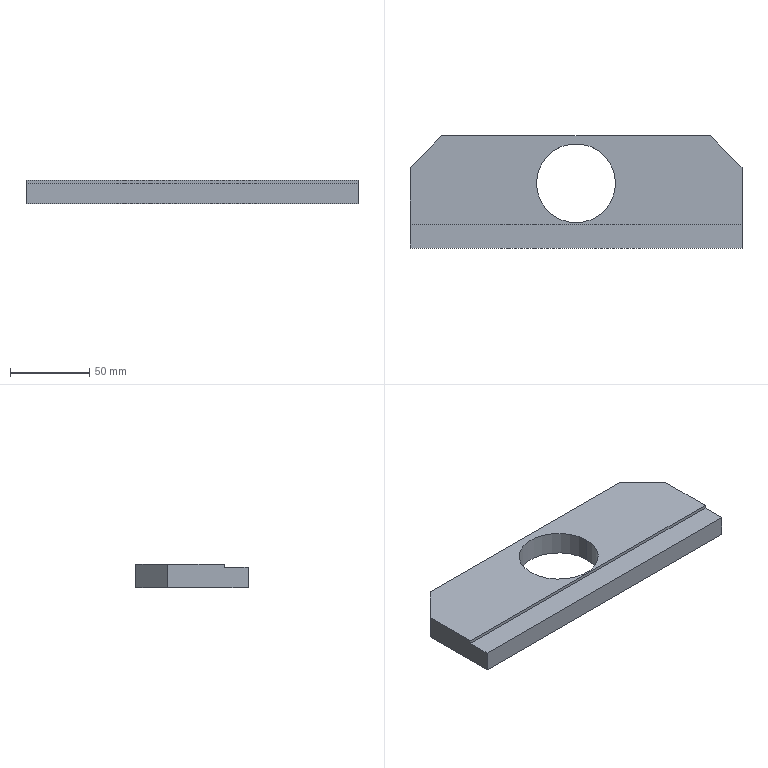Part | STEP file | 001-003-Shaft storage motor mounting plate | 1 solid | 12 faces | box 210 x 71 x 15 mm | volume 181898 mm3 | plane 10 | cylinder 2 | commonest cylinder face diameters 50 x2
STEP:
#1=CARTESIAN_POINT('',(0.,0.,0.));
#2=DIRECTION('',(0.,0.,1.));
#3=DIRECTION('',(1.,0.,0.));
#4=AXIS2_PLACEMENT_3D('',#1,#2,#3);
#5=CARTESIAN_POINT('',(-25.,5.5,15.));
#6=VERTEX_POINT('',#5);
#7=CARTESIAN_POINT('',(-25.,5.5,0.));
#8=VERTEX_POINT('',#7);
#9=CARTESIAN_POINT('',(-25.,5.5,15.));
#10=DIRECTION('',(0.,0.,-1.));
#11=VECTOR('',#10,1.);
#12=LINE('',#9,#11);
#13=CARTESIAN_POINT('',(0.,5.5,15.));
#14=DIRECTION('',(0.,0.,-1.));
#15=DIRECTION('',(-1.,0.,0.));
#16=AXIS2_PLACEMENT_3D('',#13,#14,#15);
#17=CYLINDRICAL_SURFACE('',#16,25.);
#18=CARTESIAN_POINT('',(6.283,0.));
#19=DIRECTION('',(0.,1.));
#20=VECTOR('',#19,1.);
#21=LINE('',#18,#20);
#22=(GEOMETRIC_REPRESENTATION_CONTEXT(2)PARAMETRIC_REPRESENTATION_CONTEXT()REPRESENTATION_CONTEXT('',''));
#23=DEFINITIONAL_REPRESENTATION('',(#21),#22);
#24=PCURVE('',#17,#23);
#25=CARTESIAN_POINT('',(0.,5.5,15.));
#26=DIRECTION('',(0.,0.,-1.));
#27=DIRECTION('',(-1.,0.,0.));
#28=AXIS2_PLACEMENT_3D('',#25,#26,#27);
#29=CYLINDRICAL_SURFACE('',#28,25.);
#30=CARTESIAN_POINT('',(0.,0.));
#31=DIRECTION('',(0.,1.));
#32=VECTOR('',#31,1.);
#33=LINE('',#30,#32);
#34=(GEOMETRIC_REPRESENTATION_CONTEXT(2)PARAMETRIC_REPRESENTATION_CONTEXT()REPRESENTATION_CONTEXT('',''));
#35=DEFINITIONAL_REPRESENTATION('',(#33),#34);
#36=PCURVE('',#29,#35);
#37=SURFACE_CURVE('',#12,(#24,#36),.PCURVE_S1.);
#38=EDGE_CURVE('',#6,#8,#37,.T.);
#39=ORIENTED_EDGE('',*,*,#38,.T.);
#40=CARTESIAN_POINT('',(25.,5.5,0.));
#41=VERTEX_POINT('',#40);
#42=CARTESIAN_POINT('',(0.,5.5,0.));
#43=DIRECTION('',(0.,0.,-1.));
#44=DIRECTION('',(-1.,0.,0.));
#45=AXIS2_PLACEMENT_3D('',#42,#43,#44);
#46=CIRCLE('',#45,25.);
#47=CARTESIAN_POINT('',(0.,15.));
#48=DIRECTION('',(1.,0.));
#49=VECTOR('',#48,1.);
#50=LINE('',#47,#49);
#51=(GEOMETRIC_REPRESENTATION_CONTEXT(2)PARAMETRIC_REPRESENTATION_CONTEXT()REPRESENTATION_CONTEXT('',''));
#52=DEFINITIONAL_REPRESENTATION('',(#50),#51);
#53=PCURVE('',#17,#52);
#54=CARTESIAN_POINT('',(0.,0.,0.));
#55=DIRECTION('',(0.,0.,-1.));
#56=DIRECTION('',(-1.,0.,0.));
#57=AXIS2_PLACEMENT_3D('',#54,#55,#56);
#58=PLANE('',#57);
#59=CARTESIAN_POINT('',(0.,5.5));
#60=DIRECTION('',(1.,0.));
#61=AXIS2_PLACEMENT_2D('',#59,#60);
#62=CIRCLE('',#61,25.);
#63=(GEOMETRIC_REPRESENTATION_CONTEXT(2)PARAMETRIC_REPRESENTATION_CONTEXT()REPRESENTATION_CONTEXT('',''));
#64=DEFINITIONAL_REPRESENTATION('',(#62),#63);
#65=PCURVE('',#58,#64);
#66=SURFACE_CURVE('',#46,(#53,#65),.PCURVE_S1.);
#67=EDGE_CURVE('',#41,#8,#66,.T.);
#68=ORIENTED_EDGE('',*,*,#67,.F.);
#69=CARTESIAN_POINT('',(25.,5.5,15.));
#70=VERTEX_POINT('',#69);
#71=CARTESIAN_POINT('',(25.,5.5,15.));
#72=DIRECTION('',(0.,0.,-1.));
#73=VECTOR('',#72,1.);
#74=LINE('',#71,#73);
#75=CARTESIAN_POINT('',(3.142,0.));
#76=DIRECTION('',(0.,1.));
#77=VECTOR('',#76,1.);
#78=LINE('',#75,#77);
#79=(GEOMETRIC_REPRESENTATION_CONTEXT(2)PARAMETRIC_REPRESENTATION_CONTEXT()REPRESENTATION_CONTEXT('',''));
#80=DEFINITIONAL_REPRESENTATION('',(#78),#79);
#81=PCURVE('',#17,#80);
#82=CARTESIAN_POINT('',(3.142,0.));
#83=DIRECTION('',(0.,1.));
#84=VECTOR('',#83,1.);
#85=LINE('',#82,#84);
#86=(GEOMETRIC_REPRESENTATION_CONTEXT(2)PARAMETRIC_REPRESENTATION_CONTEXT()REPRESENTATION_CONTEXT('',''));
#87=DEFINITIONAL_REPRESENTATION('',(#85),#86);
#88=PCURVE('',#29,#87);
#89=SURFACE_CURVE('',#74,(#81,#88),.PCURVE_S1.);
#90=EDGE_CURVE('',#70,#41,#89,.T.);
#91=ORIENTED_EDGE('',*,*,#90,.F.);
#92=CARTESIAN_POINT('',(0.,5.5,15.));
#93=DIRECTION('',(0.,0.,-1.));
#94=DIRECTION('',(-1.,0.,0.));
#95=AXIS2_PLACEMENT_3D('',#92,#93,#94);
#96=CIRCLE('',#95,25.);
#97=CARTESIAN_POINT('',(0.,0.));
#98=DIRECTION('',(1.,0.));
#99=VECTOR('',#98,1.);
#100=LINE('',#97,#99);
#101=(GEOMETRIC_REPRESENTATION_CONTEXT(2)PARAMETRIC_REPRESENTATION_CONTEXT()REPRESENTATION_CONTEXT('',''));
#102=DEFINITIONAL_REPRESENTATION('',(#100),#101);
#103=PCURVE('',#17,#102);
#104=CARTESIAN_POINT('',(0.,0.,15.));
#105=DIRECTION('',(0.,0.,-1.));
#106=DIRECTION('',(-1.,0.,0.));
#107=AXIS2_PLACEMENT_3D('',#104,#105,#106);
#108=PLANE('',#107);
#109=CARTESIAN_POINT('',(0.,5.5));
#110=DIRECTION('',(1.,0.));
#111=AXIS2_PLACEMENT_2D('',#109,#110);
#112=CIRCLE('',#111,25.);
#113=(GEOMETRIC_REPRESENTATION_CONTEXT(2)PARAMETRIC_REPRESENTATION_CONTEXT()REPRESENTATION_CONTEXT('',''));
#114=DEFINITIONAL_REPRESENTATION('',(#112),#113);
#115=PCURVE('',#108,#114);
#116=SURFACE_CURVE('',#96,(#103,#115),.PCURVE_S1.);
#117=EDGE_CURVE('',#70,#6,#116,.T.);
#118=ORIENTED_EDGE('',*,*,#117,.T.);
#119=EDGE_LOOP('',(#39,#68,#91,#118));
#120=FACE_BOUND('',#119,.F.);
#121=ADVANCED_FACE('',(#120),#17,.F.);
#122=CARTESIAN_POINT('',(-105.,-35.5,13.));
#123=VERTEX_POINT('',#122);
#124=CARTESIAN_POINT('',(105.,-35.5,13.));
#125=VERTEX_POINT('',#124);
#126=CARTESIAN_POINT('',(105.,-35.5,13.));
#127=DIRECTION('',(1.,0.,0.));
#128=VECTOR('',#127,1.);
#129=LINE('',#126,#128);
#130=CARTESIAN_POINT('',(-105.,-35.5,15.));
#131=DIRECTION('',(0.,1.,0.));
#132=DIRECTION('',(0.,0.,1.));
#133=AXIS2_PLACEMENT_3D('',#130,#131,#132);
#134=PLANE('',#133);
#135=CARTESIAN_POINT('',(-2.,210.));
#136=DIRECTION('',(0.,1.));
#137=VECTOR('',#136,1.);
#138=LINE('',#135,#137);
#139=(GEOMETRIC_REPRESENTATION_CONTEXT(2)PARAMETRIC_REPRESENTATION_CONTEXT()REPRESENTATION_CONTEXT('',''));
#140=DEFINITIONAL_REPRESENTATION('',(#138),#139);
#141=PCURVE('',#134,#140);
#142=CARTESIAN_POINT('',(0.,0.,13.));
#143=DIRECTION('',(0.,0.,1.));
#144=DIRECTION('',(1.,0.,0.));
#145=AXIS2_PLACEMENT_3D('',#142,#143,#144);
#146=PLANE('',#145);
#147=CARTESIAN_POINT('',(105.,-35.5));
#148=DIRECTION('',(1.,0.));
#149=VECTOR('',#148,1.);
#150=LINE('',#147,#149);
#151=(GEOMETRIC_REPRESENTATION_CONTEXT(2)PARAMETRIC_REPRESENTATION_CONTEXT()REPRESENTATION_CONTEXT('',''));
#152=DEFINITIONAL_REPRESENTATION('',(#150),#151);
#153=PCURVE('',#146,#152);
#154=SURFACE_CURVE('',#129,(#141,#153),.PCURVE_S1.);
#155=EDGE_CURVE('',#123,#125,#154,.T.);
#156=ORIENTED_EDGE('',*,*,#155,.F.);
#157=CARTESIAN_POINT('',(-105.,-35.5,0.));
#158=VERTEX_POINT('',#157);
#159=CARTESIAN_POINT('',(-105.,-35.5,15.));
#160=DIRECTION('',(0.,0.,-1.));
#161=VECTOR('',#160,1.);
#162=LINE('',#159,#161);
#163=CARTESIAN_POINT('',(0.,0.));
#164=DIRECTION('',(-1.,0.));
#165=VECTOR('',#164,1.);
#166=LINE('',#163,#165);
#167=(GEOMETRIC_REPRESENTATION_CONTEXT(2)PARAMETRIC_REPRESENTATION_CONTEXT()REPRESENTATION_CONTEXT('',''));
#168=DEFINITIONAL_REPRESENTATION('',(#166),#167);
#169=PCURVE('',#134,#168);
#170=CARTESIAN_POINT('',(-105.,-35.5,15.));
#171=DIRECTION('',(1.,0.,0.));
#172=DIRECTION('',(0.,0.,-1.));
#173=AXIS2_PLACEMENT_3D('',#170,#171,#172);
#174=PLANE('',#173);
#175=CARTESIAN_POINT('',(0.,0.));
#176=DIRECTION('',(1.,0.));
#177=VECTOR('',#176,1.);
#178=LINE('',#175,#177);
#179=(GEOMETRIC_REPRESENTATION_CONTEXT(2)PARAMETRIC_REPRESENTATION_CONTEXT()REPRESENTATION_CONTEXT('',''));
#180=DEFINITIONAL_REPRESENTATION('',(#178),#179);
#181=PCURVE('',#174,#180);
#182=SURFACE_CURVE('',#162,(#169,#181),.PCURVE_S1.);
#183=EDGE_CURVE('',#123,#158,#182,.T.);
#184=ORIENTED_EDGE('',*,*,#183,.T.);
#185=CARTESIAN_POINT('',(105.,-35.5,0.));
#186=VERTEX_POINT('',#185);
#187=CARTESIAN_POINT('',(-105.,-35.5,0.));
#188=DIRECTION('',(1.,0.,0.));
#189=VECTOR('',#188,1.);
#190=LINE('',#187,#189);
#191=CARTESIAN_POINT('',(-15.,0.));
#192=DIRECTION('',(0.,1.));
#193=VECTOR('',#192,1.);
#194=LINE('',#191,#193);
#195=(GEOMETRIC_REPRESENTATION_CONTEXT(2)PARAMETRIC_REPRESENTATION_CONTEXT()REPRESENTATION_CONTEXT('',''));
#196=DEFINITIONAL_REPRESENTATION('',(#194),#195);
#197=PCURVE('',#134,#196);
#198=CARTESIAN_POINT('',(105.,-35.5));
#199=DIRECTION('',(-1.,0.));
#200=VECTOR('',#199,1.);
#201=LINE('',#198,#200);
#202=(GEOMETRIC_REPRESENTATION_CONTEXT(2)PARAMETRIC_REPRESENTATION_CONTEXT()REPRESENTATION_CONTEXT('',''));
#203=DEFINITIONAL_REPRESENTATION('',(#201),#202);
#204=PCURVE('',#58,#203);
#205=SURFACE_CURVE('',#190,(#197,#204),.PCURVE_S1.);
#206=EDGE_CURVE('',#158,#186,#205,.T.);
#207=ORIENTED_EDGE('',*,*,#206,.T.);
#208=CARTESIAN_POINT('',(105.,-35.5,15.));
#209=DIRECTION('',(0.,0.,-1.));
#210=VECTOR('',#209,1.);
#211=LINE('',#208,#210);
#212=CARTESIAN_POINT('',(0.,210.));
#213=DIRECTION('',(-1.,0.));
#214=VECTOR('',#213,1.);
#215=LINE('',#212,#214);
#216=(GEOMETRIC_REPRESENTATION_CONTEXT(2)PARAMETRIC_REPRESENTATION_CONTEXT()REPRESENTATION_CONTEXT('',''));
#217=DEFINITIONAL_REPRESENTATION('',(#215),#216);
#218=PCURVE('',#134,#217);
#219=CARTESIAN_POINT('',(105.,-35.5,15.));
#220=DIRECTION('',(-1.,0.,0.));
#221=DIRECTION('',(0.,0.,1.));
#222=AXIS2_PLACEMENT_3D('',#219,#220,#221);
#223=PLANE('',#222);
#224=CARTESIAN_POINT('',(0.,0.));
#225=DIRECTION('',(-1.,0.));
#226=VECTOR('',#225,1.);
#227=LINE('',#224,#226);
#228=(GEOMETRIC_REPRESENTATION_CONTEXT(2)PARAMETRIC_REPRESENTATION_CONTEXT()REPRESENTATION_CONTEXT('',''));
#229=DEFINITIONAL_REPRESENTATION('',(#227),#228);
#230=PCURVE('',#223,#229);
#231=SURFACE_CURVE('',#211,(#218,#230),.PCURVE_S1.);
#232=EDGE_CURVE('',#125,#186,#231,.T.);
#233=ORIENTED_EDGE('',*,*,#232,.F.);
#234=EDGE_LOOP('',(#156,#184,#207,#233));
#235=FACE_BOUND('',#234,.T.);
#236=ADVANCED_FACE('',(#235),#134,.F.);
#237=CARTESIAN_POINT('',(105.,-20.5,15.));
#238=VERTEX_POINT('',#237);
#239=CARTESIAN_POINT('',(105.,15.5,15.));
#240=VERTEX_POINT('',#239);
#241=CARTESIAN_POINT('',(105.,-35.5,15.));
#242=DIRECTION('',(0.,1.,0.));
#243=VECTOR('',#242,1.);
#244=LINE('',#241,#243);
#245=CARTESIAN_POINT('',(0.,0.));
#246=DIRECTION('',(0.,1.));
#247=VECTOR('',#246,1.);
#248=LINE('',#245,#247);
#249=(GEOMETRIC_REPRESENTATION_CONTEXT(2)PARAMETRIC_REPRESENTATION_CONTEXT()REPRESENTATION_CONTEXT('',''));
#250=DEFINITIONAL_REPRESENTATION('',(#248),#249);
#251=PCURVE('',#223,#250);
#252=CARTESIAN_POINT('',(-105.,-35.5));
#253=DIRECTION('',(0.,1.));
#254=VECTOR('',#253,1.);
#255=LINE('',#252,#254);
#256=(GEOMETRIC_REPRESENTATION_CONTEXT(2)PARAMETRIC_REPRESENTATION_CONTEXT()REPRESENTATION_CONTEXT('',''));
#257=DEFINITIONAL_REPRESENTATION('',(#255),#256);
#258=PCURVE('',#108,#257);
#259=SURFACE_CURVE('',#244,(#251,#258),.PCURVE_S1.);
#260=EDGE_CURVE('',#238,#240,#259,.T.);
#261=ORIENTED_EDGE('',*,*,#260,.F.);
#262=CARTESIAN_POINT('',(105.,-20.5,13.));
#263=VERTEX_POINT('',#262);
#264=CARTESIAN_POINT('',(105.,-20.5,13.));
#265=DIRECTION('',(0.,0.,1.));
#266=VECTOR('',#265,1.);
#267=LINE('',#264,#266);
#268=CARTESIAN_POINT('',(-2.,15.));
#269=DIRECTION('',(1.,0.));
#270=VECTOR('',#269,1.);
#271=LINE('',#268,#270);
#272=(GEOMETRIC_REPRESENTATION_CONTEXT(2)PARAMETRIC_REPRESENTATION_CONTEXT()REPRESENTATION_CONTEXT('',''));
#273=DEFINITIONAL_REPRESENTATION('',(#271),#272);
#274=PCURVE('',#223,#273);
#275=CARTESIAN_POINT('',(105.,-20.5,13.));
#276=DIRECTION('',(0.,1.,0.));
#277=DIRECTION('',(-1.,0.,0.));
#278=AXIS2_PLACEMENT_3D('',#275,#276,#277);
#279=PLANE('',#278);
#280=CARTESIAN_POINT('',(0.,0.));
#281=DIRECTION('',(0.,1.));
#282=VECTOR('',#281,1.);
#283=LINE('',#280,#282);
#284=(GEOMETRIC_REPRESENTATION_CONTEXT(2)PARAMETRIC_REPRESENTATION_CONTEXT()REPRESENTATION_CONTEXT('',''));
#285=DEFINITIONAL_REPRESENTATION('',(#283),#284);
#286=PCURVE('',#279,#285);
#287=SURFACE_CURVE('',#267,(#274,#286),.PCURVE_S1.);
#288=EDGE_CURVE('',#263,#238,#287,.T.);
#289=ORIENTED_EDGE('',*,*,#288,.F.);
#290=CARTESIAN_POINT('',(105.,-35.5,13.));
#291=DIRECTION('',(0.,1.,0.));
#292=VECTOR('',#291,1.);
#293=LINE('',#290,#292);
#294=CARTESIAN_POINT('',(-2.,0.));
#295=DIRECTION('',(0.,1.));
#296=VECTOR('',#295,1.);
#297=LINE('',#294,#296);
#298=(GEOMETRIC_REPRESENTATION_CONTEXT(2)PARAMETRIC_REPRESENTATION_CONTEXT()REPRESENTATION_CONTEXT('',''));
#299=DEFINITIONAL_REPRESENTATION('',(#297),#298);
#300=PCURVE('',#223,#299);
#301=CARTESIAN_POINT('',(105.,-35.5));
#302=DIRECTION('',(0.,1.));
#303=VECTOR('',#302,1.);
#304=LINE('',#301,#303);
#305=(GEOMETRIC_REPRESENTATION_CONTEXT(2)PARAMETRIC_REPRESENTATION_CONTEXT()REPRESENTATION_CONTEXT('',''));
#306=DEFINITIONAL_REPRESENTATION('',(#304),#305);
#307=PCURVE('',#146,#306);
#308=SURFACE_CURVE('',#293,(#300,#307),.PCURVE_S1.);
#309=EDGE_CURVE('',#125,#263,#308,.T.);
#310=ORIENTED_EDGE('',*,*,#309,.F.);
#311=ORIENTED_EDGE('',*,*,#232,.T.);
#312=CARTESIAN_POINT('',(105.,15.5,0.));
#313=VERTEX_POINT('',#312);
#314=CARTESIAN_POINT('',(105.,-35.5,0.));
#315=DIRECTION('',(0.,1.,0.));
#316=VECTOR('',#315,1.);
#317=LINE('',#314,#316);
#318=CARTESIAN_POINT('',(-15.,0.));
#319=DIRECTION('',(0.,1.));
#320=VECTOR('',#319,1.);
#321=LINE('',#318,#320);
#322=(GEOMETRIC_REPRESENTATION_CONTEXT(2)PARAMETRIC_REPRESENTATION_CONTEXT()REPRESENTATION_CONTEXT('',''));
#323=DEFINITIONAL_REPRESENTATION('',(#321),#322);
#324=PCURVE('',#223,#323);
#325=CARTESIAN_POINT('',(-105.,-35.5));
#326=DIRECTION('',(0.,1.));
#327=VECTOR('',#326,1.);
#328=LINE('',#325,#327);
#329=(GEOMETRIC_REPRESENTATION_CONTEXT(2)PARAMETRIC_REPRESENTATION_CONTEXT()REPRESENTATION_CONTEXT('',''));
#330=DEFINITIONAL_REPRESENTATION('',(#328),#329);
#331=PCURVE('',#58,#330);
#332=SURFACE_CURVE('',#317,(#324,#331),.PCURVE_S1.);
#333=EDGE_CURVE('',#186,#313,#332,.T.);
#334=ORIENTED_EDGE('',*,*,#333,.T.);
#335=CARTESIAN_POINT('',(105.,15.5,15.));
#336=DIRECTION('',(0.,0.,1.));
#337=VECTOR('',#336,1.);
#338=LINE('',#335,#337);
#339=CARTESIAN_POINT('',(0.,51.));
#340=DIRECTION('',(1.,0.));
#341=VECTOR('',#340,1.);
#342=LINE('',#339,#341);
#343=(GEOMETRIC_REPRESENTATION_CONTEXT(2)PARAMETRIC_REPRESENTATION_CONTEXT()REPRESENTATION_CONTEXT('',''));
#344=DEFINITIONAL_REPRESENTATION('',(#342),#343);
#345=PCURVE('',#223,#344);
#346=CARTESIAN_POINT('',(85.,35.5,15.));
#347=DIRECTION('',(-0.7071,-0.7071,0.));
#348=DIRECTION('',(0.,0.,-1.));
#349=AXIS2_PLACEMENT_3D('',#346,#347,#348);
#350=PLANE('',#349);
#351=CARTESIAN_POINT('',(0.,28.284));
#352=DIRECTION('',(-1.,0.));
#353=VECTOR('',#352,1.);
#354=LINE('',#351,#353);
#355=(GEOMETRIC_REPRESENTATION_CONTEXT(2)PARAMETRIC_REPRESENTATION_CONTEXT()REPRESENTATION_CONTEXT('',''));
#356=DEFINITIONAL_REPRESENTATION('',(#354),#355);
#357=PCURVE('',#350,#356);
#358=SURFACE_CURVE('',#338,(#345,#357),.PCURVE_S1.);
#359=EDGE_CURVE('',#313,#240,#358,.T.);
#360=ORIENTED_EDGE('',*,*,#359,.T.);
#361=EDGE_LOOP('',(#261,#289,#310,#311,#334,#360));
#362=FACE_BOUND('',#361,.T.);
#363=ADVANCED_FACE('',(#362),#223,.F.);
#364=CARTESIAN_POINT('',(85.,35.5,0.));
#365=VERTEX_POINT('',#364);
#366=CARTESIAN_POINT('',(-85.,35.5,0.));
#367=VERTEX_POINT('',#366);
#368=CARTESIAN_POINT('',(-105.,35.5,0.));
#369=DIRECTION('',(-1.,0.,0.));
#370=VECTOR('',#369,1.);
#371=LINE('',#368,#370);
#372=CARTESIAN_POINT('',(-105.,35.5,15.));
#373=DIRECTION('',(0.,-1.,0.));
#374=DIRECTION('',(0.,0.,-1.));
#375=AXIS2_PLACEMENT_3D('',#372,#373,#374);
#376=PLANE('',#375);
#377=CARTESIAN_POINT('',(15.,0.));
#378=DIRECTION('',(0.,-1.));
#379=VECTOR('',#378,1.);
#380=LINE('',#377,#379);
#381=(GEOMETRIC_REPRESENTATION_CONTEXT(2)PARAMETRIC_REPRESENTATION_CONTEXT()REPRESENTATION_CONTEXT('',''));
#382=DEFINITIONAL_REPRESENTATION('',(#380),#381);
#383=PCURVE('',#376,#382);
#384=CARTESIAN_POINT('',(105.,35.5));
#385=DIRECTION('',(1.,0.));
#386=VECTOR('',#385,1.);
#387=LINE('',#384,#386);
#388=(GEOMETRIC_REPRESENTATION_CONTEXT(2)PARAMETRIC_REPRESENTATION_CONTEXT()REPRESENTATION_CONTEXT('',''));
#389=DEFINITIONAL_REPRESENTATION('',(#387),#388);
#390=PCURVE('',#58,#389);
#391=SURFACE_CURVE('',#371,(#383,#390),.PCURVE_S1.);
#392=EDGE_CURVE('',#365,#367,#391,.T.);
#393=ORIENTED_EDGE('',*,*,#392,.T.);
#394=CARTESIAN_POINT('',(-85.,35.5,15.));
#395=VERTEX_POINT('',#394);
#396=CARTESIAN_POINT('',(-85.,35.5,15.));
#397=DIRECTION('',(0.,0.,1.));
#398=VECTOR('',#397,1.);
#399=LINE('',#396,#398);
#400=CARTESIAN_POINT('',(0.,20.));
#401=DIRECTION('',(-1.,0.));
#402=VECTOR('',#401,1.);
#403=LINE('',#400,#402);
#404=(GEOMETRIC_REPRESENTATION_CONTEXT(2)PARAMETRIC_REPRESENTATION_CONTEXT()REPRESENTATION_CONTEXT('',''));
#405=DEFINITIONAL_REPRESENTATION('',(#403),#404);
#406=PCURVE('',#376,#405);
#407=CARTESIAN_POINT('',(-105.,15.5,15.));
#408=DIRECTION('',(0.7071,-0.7071,0.));
#409=DIRECTION('',(0.,0.,-1.));
#410=AXIS2_PLACEMENT_3D('',#407,#408,#409);
#411=PLANE('',#410);
#412=CARTESIAN_POINT('',(0.,28.284));
#413=DIRECTION('',(-1.,0.));
#414=VECTOR('',#413,1.);
#415=LINE('',#412,#414);
#416=(GEOMETRIC_REPRESENTATION_CONTEXT(2)PARAMETRIC_REPRESENTATION_CONTEXT()REPRESENTATION_CONTEXT('',''));
#417=DEFINITIONAL_REPRESENTATION('',(#415),#416);
#418=PCURVE('',#411,#417);
#419=SURFACE_CURVE('',#399,(#406,#418),.PCURVE_S1.);
#420=EDGE_CURVE('',#367,#395,#419,.T.);
#421=ORIENTED_EDGE('',*,*,#420,.T.);
#422=CARTESIAN_POINT('',(85.,35.5,15.));
#423=VERTEX_POINT('',#422);
#424=CARTESIAN_POINT('',(-105.,35.5,15.));
#425=DIRECTION('',(-1.,0.,0.));
#426=VECTOR('',#425,1.);
#427=LINE('',#424,#426);
#428=CARTESIAN_POINT('',(0.,0.));
#429=DIRECTION('',(0.,-1.));
#430=VECTOR('',#429,1.);
#431=LINE('',#428,#430);
#432=(GEOMETRIC_REPRESENTATION_CONTEXT(2)PARAMETRIC_REPRESENTATION_CONTEXT()REPRESENTATION_CONTEXT('',''));
#433=DEFINITIONAL_REPRESENTATION('',(#431),#432);
#434=PCURVE('',#376,#433);
#435=CARTESIAN_POINT('',(105.,35.5));
#436=DIRECTION('',(1.,0.));
#437=VECTOR('',#436,1.);
#438=LINE('',#435,#437);
#439=(GEOMETRIC_REPRESENTATION_CONTEXT(2)PARAMETRIC_REPRESENTATION_CONTEXT()REPRESENTATION_CONTEXT('',''));
#440=DEFINITIONAL_REPRESENTATION('',(#438),#439);
#441=PCURVE('',#108,#440);
#442=SURFACE_CURVE('',#427,(#434,#441),.PCURVE_S1.);
#443=EDGE_CURVE('',#423,#395,#442,.T.);
#444=ORIENTED_EDGE('',*,*,#443,.F.);
#445=CARTESIAN_POINT('',(85.,35.5,15.));
#446=DIRECTION('',(0.,0.,-1.));
#447=VECTOR('',#446,1.);
#448=LINE('',#445,#447);
#449=CARTESIAN_POINT('',(0.,190.));
#450=DIRECTION('',(1.,0.));
#451=VECTOR('',#450,1.);
#452=LINE('',#449,#451);
#453=(GEOMETRIC_REPRESENTATION_CONTEXT(2)PARAMETRIC_REPRESENTATION_CONTEXT()REPRESENTATION_CONTEXT('',''));
#454=DEFINITIONAL_REPRESENTATION('',(#452),#453);
#455=PCURVE('',#376,#454);
#456=CARTESIAN_POINT('',(0.,0.));
#457=DIRECTION('',(1.,0.));
#458=VECTOR('',#457,1.);
#459=LINE('',#456,#458);
#460=(GEOMETRIC_REPRESENTATION_CONTEXT(2)PARAMETRIC_REPRESENTATION_CONTEXT()REPRESENTATION_CONTEXT('',''));
#461=DEFINITIONAL_REPRESENTATION('',(#459),#460);
#462=PCURVE('',#350,#461);
#463=SURFACE_CURVE('',#448,(#455,#462),.PCURVE_S1.);
#464=EDGE_CURVE('',#423,#365,#463,.T.);
#465=ORIENTED_EDGE('',*,*,#464,.T.);
#466=EDGE_LOOP('',(#393,#421,#444,#465));
#467=FACE_BOUND('',#466,.T.);
#468=ADVANCED_FACE('',(#467),#376,.F.);
#469=CARTESIAN_POINT('',(-105.,-20.5,13.));
#470=VERTEX_POINT('',#469);
#471=CARTESIAN_POINT('',(-105.,-35.5,13.));
#472=DIRECTION('',(0.,-1.,0.));
#473=VECTOR('',#472,1.);
#474=LINE('',#471,#473);
#475=CARTESIAN_POINT('',(2.,0.));
#476=DIRECTION('',(0.,-1.));
#477=VECTOR('',#476,1.);
#478=LINE('',#475,#477);
#479=(GEOMETRIC_REPRESENTATION_CONTEXT(2)PARAMETRIC_REPRESENTATION_CONTEXT()REPRESENTATION_CONTEXT('',''));
#480=DEFINITIONAL_REPRESENTATION('',(#478),#479);
#481=PCURVE('',#174,#480);
#482=CARTESIAN_POINT('',(-105.,-35.5));
#483=DIRECTION('',(0.,-1.));
#484=VECTOR('',#483,1.);
#485=LINE('',#482,#484);
#486=(GEOMETRIC_REPRESENTATION_CONTEXT(2)PARAMETRIC_REPRESENTATION_CONTEXT()REPRESENTATION_CONTEXT('',''));
#487=DEFINITIONAL_REPRESENTATION('',(#485),#486);
#488=PCURVE('',#146,#487);
#489=SURFACE_CURVE('',#474,(#481,#488),.PCURVE_S1.);
#490=EDGE_CURVE('',#470,#123,#489,.T.);
#491=ORIENTED_EDGE('',*,*,#490,.F.);
#492=CARTESIAN_POINT('',(-105.,-20.5,15.));
#493=VERTEX_POINT('',#492);
#494=CARTESIAN_POINT('',(-105.,-20.5,13.));
#495=DIRECTION('',(0.,0.,1.));
#496=VECTOR('',#495,1.);
#497=LINE('',#494,#496);
#498=CARTESIAN_POINT('',(2.,15.));
#499=DIRECTION('',(-1.,0.));
#500=VECTOR('',#499,1.);
#501=LINE('',#498,#500);
#502=(GEOMETRIC_REPRESENTATION_CONTEXT(2)PARAMETRIC_REPRESENTATION_CONTEXT()REPRESENTATION_CONTEXT('',''));
#503=DEFINITIONAL_REPRESENTATION('',(#501),#502);
#504=PCURVE('',#174,#503);
#505=CARTESIAN_POINT('',(210.,0.));
#506=DIRECTION('',(0.,1.));
#507=VECTOR('',#506,1.);
#508=LINE('',#505,#507);
#509=(GEOMETRIC_REPRESENTATION_CONTEXT(2)PARAMETRIC_REPRESENTATION_CONTEXT()REPRESENTATION_CONTEXT('',''));
#510=DEFINITIONAL_REPRESENTATION('',(#508),#509);
#511=PCURVE('',#279,#510);
#512=SURFACE_CURVE('',#497,(#504,#511),.PCURVE_S1.);
#513=EDGE_CURVE('',#470,#493,#512,.T.);
#514=ORIENTED_EDGE('',*,*,#513,.T.);
#515=CARTESIAN_POINT('',(-105.,15.5,15.));
#516=VERTEX_POINT('',#515);
#517=CARTESIAN_POINT('',(-105.,-35.5,15.));
#518=DIRECTION('',(0.,-1.,0.));
#519=VECTOR('',#518,1.);
#520=LINE('',#517,#519);
#521=CARTESIAN_POINT('',(0.,0.));
#522=DIRECTION('',(0.,-1.));
#523=VECTOR('',#522,1.);
#524=LINE('',#521,#523);
#525=(GEOMETRIC_REPRESENTATION_CONTEXT(2)PARAMETRIC_REPRESENTATION_CONTEXT()REPRESENTATION_CONTEXT('',''));
#526=DEFINITIONAL_REPRESENTATION('',(#524),#525);
#527=PCURVE('',#174,#526);
#528=CARTESIAN_POINT('',(105.,-35.5));
#529=DIRECTION('',(0.,-1.));
#530=VECTOR('',#529,1.);
#531=LINE('',#528,#530);
#532=(GEOMETRIC_REPRESENTATION_CONTEXT(2)PARAMETRIC_REPRESENTATION_CONTEXT()REPRESENTATION_CONTEXT('',''));
#533=DEFINITIONAL_REPRESENTATION('',(#531),#532);
#534=PCURVE('',#108,#533);
#535=SURFACE_CURVE('',#520,(#527,#534),.PCURVE_S1.);
#536=EDGE_CURVE('',#516,#493,#535,.T.);
#537=ORIENTED_EDGE('',*,*,#536,.F.);
#538=CARTESIAN_POINT('',(-105.,15.5,0.));
#539=VERTEX_POINT('',#538);
#540=CARTESIAN_POINT('',(-105.,15.5,15.));
#541=DIRECTION('',(0.,0.,-1.));
#542=VECTOR('',#541,1.);
#543=LINE('',#540,#542);
#544=CARTESIAN_POINT('',(0.,51.));
#545=DIRECTION('',(1.,0.));
#546=VECTOR('',#545,1.);
#547=LINE('',#544,#546);
#548=(GEOMETRIC_REPRESENTATION_CONTEXT(2)PARAMETRIC_REPRESENTATION_CONTEXT()REPRESENTATION_CONTEXT('',''));
#549=DEFINITIONAL_REPRESENTATION('',(#547),#548);
#550=PCURVE('',#174,#549);
#551=CARTESIAN_POINT('',(0.,0.));
#552=DIRECTION('',(1.,0.));
#553=VECTOR('',#552,1.);
#554=LINE('',#551,#553);
#555=(GEOMETRIC_REPRESENTATION_CONTEXT(2)PARAMETRIC_REPRESENTATION_CONTEXT()REPRESENTATION_CONTEXT('',''));
#556=DEFINITIONAL_REPRESENTATION('',(#554),#555);
#557=PCURVE('',#411,#556);
#558=SURFACE_CURVE('',#543,(#550,#557),.PCURVE_S1.);
#559=EDGE_CURVE('',#516,#539,#558,.T.);
#560=ORIENTED_EDGE('',*,*,#559,.T.);
#561=CARTESIAN_POINT('',(-105.,-35.5,0.));
#562=DIRECTION('',(0.,-1.,0.));
#563=VECTOR('',#562,1.);
#564=LINE('',#561,#563);
#565=CARTESIAN_POINT('',(15.,0.));
#566=DIRECTION('',(0.,-1.));
#567=VECTOR('',#566,1.);
#568=LINE('',#565,#567);
#569=(GEOMETRIC_REPRESENTATION_CONTEXT(2)PARAMETRIC_REPRESENTATION_CONTEXT()REPRESENTATION_CONTEXT('',''));
#570=DEFINITIONAL_REPRESENTATION('',(#568),#569);
#571=PCURVE('',#174,#570);
#572=CARTESIAN_POINT('',(105.,-35.5));
#573=DIRECTION('',(0.,-1.));
#574=VECTOR('',#573,1.);
#575=LINE('',#572,#574);
#576=(GEOMETRIC_REPRESENTATION_CONTEXT(2)PARAMETRIC_REPRESENTATION_CONTEXT()REPRESENTATION_CONTEXT('',''));
#577=DEFINITIONAL_REPRESENTATION('',(#575),#576);
#578=PCURVE('',#58,#577);
#579=SURFACE_CURVE('',#564,(#571,#578),.PCURVE_S1.);
#580=EDGE_CURVE('',#539,#158,#579,.T.);
#581=ORIENTED_EDGE('',*,*,#580,.T.);
#582=ORIENTED_EDGE('',*,*,#183,.F.);
#583=EDGE_LOOP('',(#491,#514,#537,#560,#581,#582));
#584=FACE_BOUND('',#583,.T.);
#585=ADVANCED_FACE('',(#584),#174,.F.);
#586=CARTESIAN_POINT('',(0.,5.5,15.));
#587=DIRECTION('',(0.,0.,-1.));
#588=DIRECTION('',(-1.,0.,0.));
#589=AXIS2_PLACEMENT_3D('',#586,#587,#588);
#590=CIRCLE('',#589,25.);
#591=CARTESIAN_POINT('',(0.,5.5));
#592=DIRECTION('',(1.,0.));
#593=AXIS2_PLACEMENT_2D('',#591,#592);
#594=CIRCLE('',#593,25.);
#595=(GEOMETRIC_REPRESENTATION_CONTEXT(2)PARAMETRIC_REPRESENTATION_CONTEXT()REPRESENTATION_CONTEXT('',''));
#596=DEFINITIONAL_REPRESENTATION('',(#594),#595);
#597=PCURVE('',#108,#596);
#598=CARTESIAN_POINT('',(0.,0.));
#599=DIRECTION('',(1.,0.));
#600=VECTOR('',#599,1.);
#601=LINE('',#598,#600);
#602=(GEOMETRIC_REPRESENTATION_CONTEXT(2)PARAMETRIC_REPRESENTATION_CONTEXT()REPRESENTATION_CONTEXT('',''));
#603=DEFINITIONAL_REPRESENTATION('',(#601),#602);
#604=PCURVE('',#29,#603);
#605=SURFACE_CURVE('',#590,(#597,#604),.PCURVE_S1.);
#606=EDGE_CURVE('',#6,#70,#605,.T.);
#607=ORIENTED_EDGE('',*,*,#606,.T.);
#608=ORIENTED_EDGE('',*,*,#117,.T.);
#609=EDGE_LOOP('',(#607,#608));
#610=FACE_BOUND('',#609,.T.);
#611=ORIENTED_EDGE('',*,*,#536,.T.);
#612=CARTESIAN_POINT('',(105.,-20.5,15.));
#613=DIRECTION('',(-1.,0.,0.));
#614=VECTOR('',#613,1.);
#615=LINE('',#612,#614);
#616=CARTESIAN_POINT('',(-105.,-20.5));
#617=DIRECTION('',(1.,0.));
#618=VECTOR('',#617,1.);
#619=LINE('',#616,#618);
#620=(GEOMETRIC_REPRESENTATION_CONTEXT(2)PARAMETRIC_REPRESENTATION_CONTEXT()REPRESENTATION_CONTEXT('',''));
#621=DEFINITIONAL_REPRESENTATION('',(#619),#620);
#622=PCURVE('',#108,#621);
#623=CARTESIAN_POINT('',(0.,2.));
#624=DIRECTION('',(1.,0.));
#625=VECTOR('',#624,1.);
#626=LINE('',#623,#625);
#627=(GEOMETRIC_REPRESENTATION_CONTEXT(2)PARAMETRIC_REPRESENTATION_CONTEXT()REPRESENTATION_CONTEXT('',''));
#628=DEFINITIONAL_REPRESENTATION('',(#626),#627);
#629=PCURVE('',#279,#628);
#630=SURFACE_CURVE('',#615,(#622,#629),.PCURVE_S1.);
#631=EDGE_CURVE('',#238,#493,#630,.T.);
#632=ORIENTED_EDGE('',*,*,#631,.F.);
#633=ORIENTED_EDGE('',*,*,#260,.T.);
#634=CARTESIAN_POINT('',(85.,35.5,15.));
#635=DIRECTION('',(-0.7071,0.7071,0.));
#636=VECTOR('',#635,1.);
#637=LINE('',#634,#636);
#638=CARTESIAN_POINT('',(-85.,35.5));
#639=DIRECTION('',(0.7071,0.7071));
#640=VECTOR('',#639,1.);
#641=LINE('',#638,#640);
#642=(GEOMETRIC_REPRESENTATION_CONTEXT(2)PARAMETRIC_REPRESENTATION_CONTEXT()REPRESENTATION_CONTEXT('',''));
#643=DEFINITIONAL_REPRESENTATION('',(#641),#642);
#644=PCURVE('',#108,#643);
#645=CARTESIAN_POINT('',(0.,0.));
#646=DIRECTION('',(0.,-1.));
#647=VECTOR('',#646,1.);
#648=LINE('',#645,#647);
#649=(GEOMETRIC_REPRESENTATION_CONTEXT(2)PARAMETRIC_REPRESENTATION_CONTEXT()REPRESENTATION_CONTEXT('',''));
#650=DEFINITIONAL_REPRESENTATION('',(#648),#649);
#651=PCURVE('',#350,#650);
#652=SURFACE_CURVE('',#637,(#644,#651),.PCURVE_S1.);
#653=EDGE_CURVE('',#240,#423,#652,.T.);
#654=ORIENTED_EDGE('',*,*,#653,.T.);
#655=ORIENTED_EDGE('',*,*,#443,.T.);
#656=CARTESIAN_POINT('',(-105.,15.5,15.));
#657=DIRECTION('',(-0.7071,-0.7071,0.));
#658=VECTOR('',#657,1.);
#659=LINE('',#656,#658);
#660=CARTESIAN_POINT('',(105.,15.5));
#661=DIRECTION('',(0.7071,-0.7071));
#662=VECTOR('',#661,1.);
#663=LINE('',#660,#662);
#664=(GEOMETRIC_REPRESENTATION_CONTEXT(2)PARAMETRIC_REPRESENTATION_CONTEXT()REPRESENTATION_CONTEXT('',''));
#665=DEFINITIONAL_REPRESENTATION('',(#663),#664);
#666=PCURVE('',#108,#665);
#667=CARTESIAN_POINT('',(0.,0.));
#668=DIRECTION('',(0.,-1.));
#669=VECTOR('',#668,1.);
#670=LINE('',#667,#669);
#671=(GEOMETRIC_REPRESENTATION_CONTEXT(2)PARAMETRIC_REPRESENTATION_CONTEXT()REPRESENTATION_CONTEXT('',''));
#672=DEFINITIONAL_REPRESENTATION('',(#670),#671);
#673=PCURVE('',#411,#672);
#674=SURFACE_CURVE('',#659,(#666,#673),.PCURVE_S1.);
#675=EDGE_CURVE('',#395,#516,#674,.T.);
#676=ORIENTED_EDGE('',*,*,#675,.T.);
#677=EDGE_LOOP('',(#611,#632,#633,#654,#655,#676));
#678=FACE_BOUND('',#677,.T.);
#679=ADVANCED_FACE('',(#610,#678),#108,.F.);
#680=CARTESIAN_POINT('',(0.,5.5,0.));
#681=DIRECTION('',(0.,0.,-1.));
#682=DIRECTION('',(-1.,0.,0.));
#683=AXIS2_PLACEMENT_3D('',#680,#681,#682);
#684=CIRCLE('',#683,25.);
#685=CARTESIAN_POINT('',(0.,5.5));
#686=DIRECTION('',(1.,0.));
#687=AXIS2_PLACEMENT_2D('',#685,#686);
#688=CIRCLE('',#687,25.);
#689=(GEOMETRIC_REPRESENTATION_CONTEXT(2)PARAMETRIC_REPRESENTATION_CONTEXT()REPRESENTATION_CONTEXT('',''));
#690=DEFINITIONAL_REPRESENTATION('',(#688),#689);
#691=PCURVE('',#58,#690);
#692=CARTESIAN_POINT('',(0.,15.));
#693=DIRECTION('',(1.,0.));
#694=VECTOR('',#693,1.);
#695=LINE('',#692,#694);
#696=(GEOMETRIC_REPRESENTATION_CONTEXT(2)PARAMETRIC_REPRESENTATION_CONTEXT()REPRESENTATION_CONTEXT('',''));
#697=DEFINITIONAL_REPRESENTATION('',(#695),#696);
#698=PCURVE('',#29,#697);
#699=SURFACE_CURVE('',#684,(#691,#698),.PCURVE_S1.);
#700=EDGE_CURVE('',#8,#41,#699,.T.);
#701=ORIENTED_EDGE('',*,*,#700,.F.);
#702=ORIENTED_EDGE('',*,*,#67,.F.);
#703=EDGE_LOOP('',(#701,#702));
#704=FACE_BOUND('',#703,.T.);
#705=ORIENTED_EDGE('',*,*,#580,.F.);
#706=CARTESIAN_POINT('',(-60.25,60.25,0.));
#707=DIRECTION('',(0.7071,0.7071,0.));
#708=VECTOR('',#707,1.);
#709=LINE('',#706,#708);
#710=CARTESIAN_POINT('',(60.25,60.25));
#711=DIRECTION('',(-0.7071,0.7071));
#712=VECTOR('',#711,1.);
#713=LINE('',#710,#712);
#714=(GEOMETRIC_REPRESENTATION_CONTEXT(2)PARAMETRIC_REPRESENTATION_CONTEXT()REPRESENTATION_CONTEXT('',''));
#715=DEFINITIONAL_REPRESENTATION('',(#713),#714);
#716=PCURVE('',#58,#715);
#717=CARTESIAN_POINT('',(15.,63.286));
#718=DIRECTION('',(0.,1.));
#719=VECTOR('',#718,1.);
#720=LINE('',#717,#719);
#721=(GEOMETRIC_REPRESENTATION_CONTEXT(2)PARAMETRIC_REPRESENTATION_CONTEXT()REPRESENTATION_CONTEXT('',''));
#722=DEFINITIONAL_REPRESENTATION('',(#720),#721);
#723=PCURVE('',#411,#722);
#724=SURFACE_CURVE('',#709,(#716,#723),.PCURVE_S1.);
#725=EDGE_CURVE('',#539,#367,#724,.T.);
#726=ORIENTED_EDGE('',*,*,#725,.T.);
#727=ORIENTED_EDGE('',*,*,#392,.F.);
#728=CARTESIAN_POINT('',(60.25,60.25,0.));
#729=DIRECTION('',(0.7071,-0.7071,0.));
#730=VECTOR('',#729,1.);
#731=LINE('',#728,#730);
#732=CARTESIAN_POINT('',(-60.25,60.25));
#733=DIRECTION('',(-0.7071,-0.7071));
#734=VECTOR('',#733,1.);
#735=LINE('',#732,#734);
#736=(GEOMETRIC_REPRESENTATION_CONTEXT(2)PARAMETRIC_REPRESENTATION_CONTEXT()REPRESENTATION_CONTEXT('',''));
#737=DEFINITIONAL_REPRESENTATION('',(#735),#736);
#738=PCURVE('',#58,#737);
#739=CARTESIAN_POINT('',(15.,-35.002));
#740=DIRECTION('',(0.,1.));
#741=VECTOR('',#740,1.);
#742=LINE('',#739,#741);
#743=(GEOMETRIC_REPRESENTATION_CONTEXT(2)PARAMETRIC_REPRESENTATION_CONTEXT()REPRESENTATION_CONTEXT('',''));
#744=DEFINITIONAL_REPRESENTATION('',(#742),#743);
#745=PCURVE('',#350,#744);
#746=SURFACE_CURVE('',#731,(#738,#745),.PCURVE_S1.);
#747=EDGE_CURVE('',#365,#313,#746,.T.);
#748=ORIENTED_EDGE('',*,*,#747,.T.);
#749=ORIENTED_EDGE('',*,*,#333,.F.);
#750=ORIENTED_EDGE('',*,*,#206,.F.);
#751=EDGE_LOOP('',(#705,#726,#727,#748,#749,#750));
#752=FACE_BOUND('',#751,.T.);
#753=ADVANCED_FACE('',(#704,#752),#58,.T.);
#754=ORIENTED_EDGE('',*,*,#675,.F.);
#755=ORIENTED_EDGE('',*,*,#420,.F.);
#756=ORIENTED_EDGE('',*,*,#725,.F.);
#757=ORIENTED_EDGE('',*,*,#559,.F.);
#758=EDGE_LOOP('',(#754,#755,#756,#757));
#759=FACE_BOUND('',#758,.T.);
#760=ADVANCED_FACE('',(#759),#411,.F.);
#761=ORIENTED_EDGE('',*,*,#653,.F.);
#762=ORIENTED_EDGE('',*,*,#359,.F.);
#763=ORIENTED_EDGE('',*,*,#747,.F.);
#764=ORIENTED_EDGE('',*,*,#464,.F.);
#765=EDGE_LOOP('',(#761,#762,#763,#764));
#766=FACE_BOUND('',#765,.T.);
#767=ADVANCED_FACE('',(#766),#350,.F.);
#768=ORIENTED_EDGE('',*,*,#631,.T.);
#769=ORIENTED_EDGE('',*,*,#513,.F.);
#770=CARTESIAN_POINT('',(105.,-20.5,13.));
#771=DIRECTION('',(-1.,0.,0.));
#772=VECTOR('',#771,1.);
#773=LINE('',#770,#772);
#774=CARTESIAN_POINT('',(0.,0.));
#775=DIRECTION('',(1.,0.));
#776=VECTOR('',#775,1.);
#777=LINE('',#774,#776);
#778=(GEOMETRIC_REPRESENTATION_CONTEXT(2)PARAMETRIC_REPRESENTATION_CONTEXT()REPRESENTATION_CONTEXT('',''));
#779=DEFINITIONAL_REPRESENTATION('',(#777),#778);
#780=PCURVE('',#279,#779);
#781=CARTESIAN_POINT('',(105.,-20.5));
#782=DIRECTION('',(-1.,0.));
#783=VECTOR('',#782,1.);
#784=LINE('',#781,#783);
#785=(GEOMETRIC_REPRESENTATION_CONTEXT(2)PARAMETRIC_REPRESENTATION_CONTEXT()REPRESENTATION_CONTEXT('',''));
#786=DEFINITIONAL_REPRESENTATION('',(#784),#785);
#787=PCURVE('',#146,#786);
#788=SURFACE_CURVE('',#773,(#780,#787),.PCURVE_S1.);
#789=EDGE_CURVE('',#263,#470,#788,.T.);
#790=ORIENTED_EDGE('',*,*,#789,.F.);
#791=ORIENTED_EDGE('',*,*,#288,.T.);
#792=EDGE_LOOP('',(#768,#769,#790,#791));
#793=FACE_BOUND('',#792,.T.);
#794=ADVANCED_FACE('',(#793),#279,.F.);
#795=ORIENTED_EDGE('',*,*,#309,.T.);
#796=ORIENTED_EDGE('',*,*,#789,.T.);
#797=ORIENTED_EDGE('',*,*,#490,.T.);
#798=ORIENTED_EDGE('',*,*,#155,.T.);
#799=EDGE_LOOP('',(#795,#796,#797,#798));
#800=FACE_BOUND('',#799,.T.);
#801=ADVANCED_FACE('',(#800),#146,.T.);
#802=ORIENTED_EDGE('',*,*,#700,.F.);
#803=ORIENTED_EDGE('',*,*,#38,.F.);
#804=ORIENTED_EDGE('',*,*,#606,.T.);
#805=ORIENTED_EDGE('',*,*,#90,.T.);
#806=EDGE_LOOP('',(#802,#803,#804,#805));
#807=FACE_BOUND('',#806,.F.);
#808=ADVANCED_FACE('',(#807),#29,.F.);
#809=CLOSED_SHELL('',(#121,#236,#363,#468,#585,#679,#753,#760,#767,#794,#801,#808));
#810=MANIFOLD_SOLID_BREP('',#809);
#811=(LENGTH_UNIT()NAMED_UNIT(*)SI_UNIT(.MILLI.,.METRE.));
#812=UNCERTAINTY_MEASURE_WITH_UNIT(LENGTH_MEASURE(0.0000001),#811,'','');
#813=(NAMED_UNIT(*)PLANE_ANGLE_UNIT()SI_UNIT($,.RADIAN.));
#814=(NAMED_UNIT(*)SI_UNIT($,.STERADIAN.)SOLID_ANGLE_UNIT());
#815=(GEOMETRIC_REPRESENTATION_CONTEXT(3)GLOBAL_UNCERTAINTY_ASSIGNED_CONTEXT((#812))GLOBAL_UNIT_ASSIGNED_CONTEXT((#811,#813,#814))REPRESENTATION_CONTEXT('',''));
#816=ADVANCED_BREP_SHAPE_REPRESENTATION('',(#4,#810),#815);